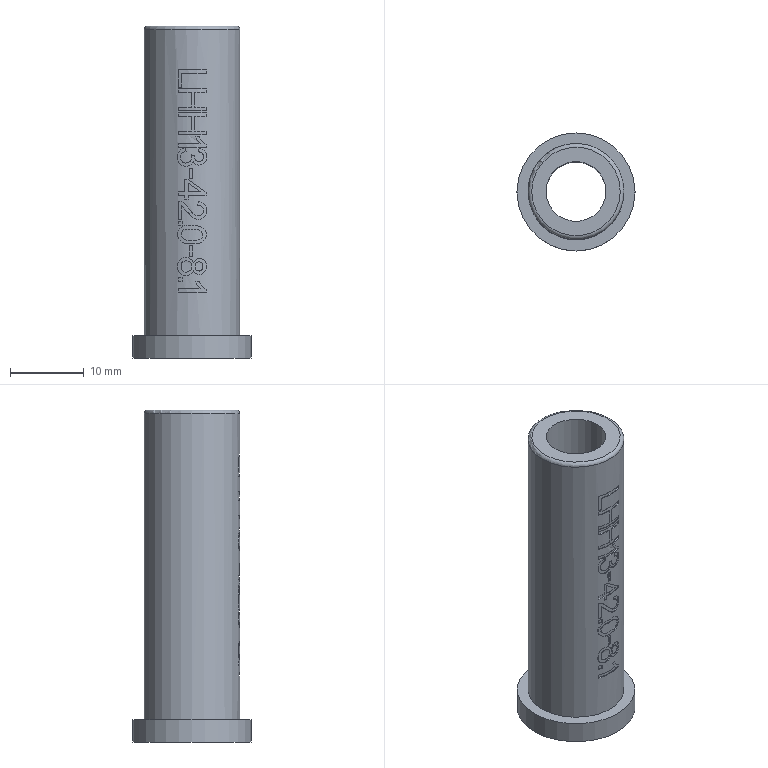Part | STEP file | PN_0056_id1706_x_t | 1 solid | 155 faces | box 16 x 16 x 45 mm | volume 3853 mm3 | plane 99 | cylinder 55 | torus 1 | commonest cylinder face diameters 12.8 x14 13 x5 1.231 x2 1.539 x2 2.242 x2 4.739 x2